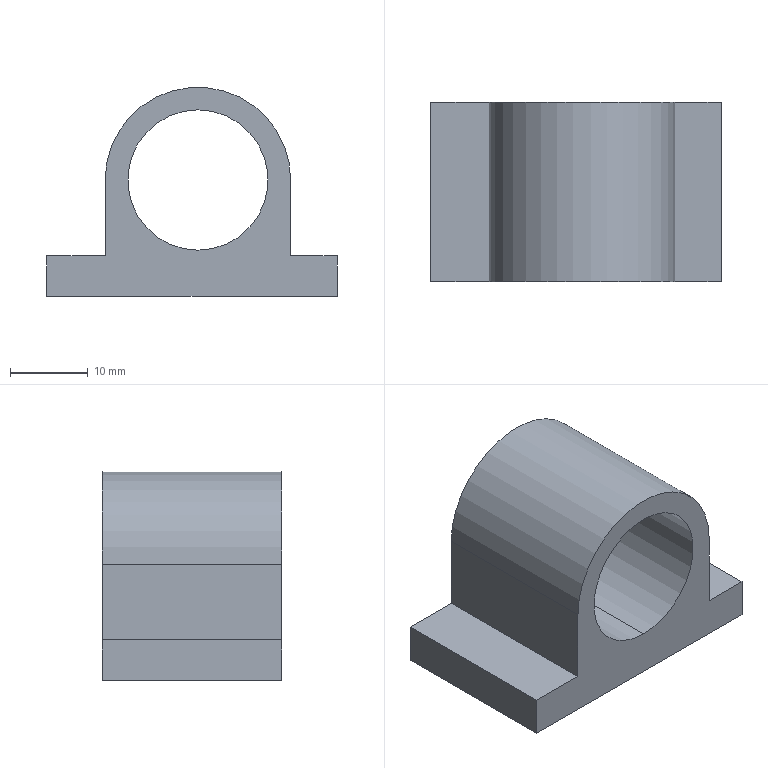Part | STEP file | 1 solid | 12 faces | box 37.23 x 23 x 26.824 mm | volume 9039 mm3 | plane 9 | cylinder 3 | commonest cylinder face diameters 18 x2 23.807 x1
STEP:
#1=CARTESIAN_POINT('',(0.,0.,0.));
#2=DIRECTION('',(0.,0.,1.));
#3=DIRECTION('',(1.,0.,0.));
#4=AXIS2_PLACEMENT_3D('',#1,#2,#3);
#5=CARTESIAN_POINT('',(340.649,373.299,152.933));
#6=VERTEX_POINT('',#5);
#7=CARTESIAN_POINT('',(340.649,350.299,152.933));
#8=VERTEX_POINT('',#7);
#9=CARTESIAN_POINT('',(340.649,373.299,152.933));
#10=DIRECTION('',(0.,-1.,0.));
#11=VECTOR('',#10,1.);
#12=LINE('',#9,#11);
#13=CARTESIAN_POINT('',(340.649,373.299,161.933));
#14=DIRECTION('',(0.,-1.,0.));
#15=DIRECTION('',(0.,0.,-1.));
#16=AXIS2_PLACEMENT_3D('',#13,#14,#15);
#17=CYLINDRICAL_SURFACE('',#16,9.);
#18=CARTESIAN_POINT('',(6.283,0.));
#19=DIRECTION('',(0.,1.));
#20=VECTOR('',#19,1.);
#21=LINE('',#18,#20);
#22=(GEOMETRIC_REPRESENTATION_CONTEXT(2)PARAMETRIC_REPRESENTATION_CONTEXT()REPRESENTATION_CONTEXT('',''));
#23=DEFINITIONAL_REPRESENTATION('',(#21),#22);
#24=PCURVE('',#17,#23);
#25=CARTESIAN_POINT('',(340.649,373.299,161.933));
#26=DIRECTION('',(0.,-1.,0.));
#27=DIRECTION('',(0.,0.,-1.));
#28=AXIS2_PLACEMENT_3D('',#25,#26,#27);
#29=CYLINDRICAL_SURFACE('',#28,9.);
#30=CARTESIAN_POINT('',(0.,0.));
#31=DIRECTION('',(0.,1.));
#32=VECTOR('',#31,1.);
#33=LINE('',#30,#32);
#34=(GEOMETRIC_REPRESENTATION_CONTEXT(2)PARAMETRIC_REPRESENTATION_CONTEXT()REPRESENTATION_CONTEXT('',''));
#35=DEFINITIONAL_REPRESENTATION('',(#33),#34);
#36=PCURVE('',#29,#35);
#37=SURFACE_CURVE('',#12,(#24,#36),.PCURVE_S1.);
#38=EDGE_CURVE('',#6,#8,#37,.T.);
#39=ORIENTED_EDGE('',*,*,#38,.T.);
#40=CARTESIAN_POINT('',(340.649,350.299,170.933));
#41=VERTEX_POINT('',#40);
#42=CARTESIAN_POINT('',(340.649,350.299,161.933));
#43=DIRECTION('',(0.,-1.,0.));
#44=DIRECTION('',(0.,0.,-1.));
#45=AXIS2_PLACEMENT_3D('',#42,#43,#44);
#46=CIRCLE('',#45,9.);
#47=CARTESIAN_POINT('',(0.,23.));
#48=DIRECTION('',(1.,0.));
#49=VECTOR('',#48,1.);
#50=LINE('',#47,#49);
#51=(GEOMETRIC_REPRESENTATION_CONTEXT(2)PARAMETRIC_REPRESENTATION_CONTEXT()REPRESENTATION_CONTEXT('',''));
#52=DEFINITIONAL_REPRESENTATION('',(#50),#51);
#53=PCURVE('',#17,#52);
#54=CARTESIAN_POINT('',(340.649,350.299,161.933));
#55=DIRECTION('',(0.,-1.,0.));
#56=DIRECTION('',(0.,0.,-1.));
#57=AXIS2_PLACEMENT_3D('',#54,#55,#56);
#58=PLANE('',#57);
#59=CARTESIAN_POINT('',(0.,0.));
#60=DIRECTION('',(1.,0.));
#61=AXIS2_PLACEMENT_2D('',#59,#60);
#62=CIRCLE('',#61,9.);
#63=(GEOMETRIC_REPRESENTATION_CONTEXT(2)PARAMETRIC_REPRESENTATION_CONTEXT()REPRESENTATION_CONTEXT('',''));
#64=DEFINITIONAL_REPRESENTATION('',(#62),#63);
#65=PCURVE('',#58,#64);
#66=SURFACE_CURVE('',#46,(#53,#65),.PCURVE_S1.);
#67=EDGE_CURVE('',#41,#8,#66,.T.);
#68=ORIENTED_EDGE('',*,*,#67,.F.);
#69=CARTESIAN_POINT('',(340.649,373.299,170.933));
#70=VERTEX_POINT('',#69);
#71=CARTESIAN_POINT('',(340.649,373.299,170.933));
#72=DIRECTION('',(0.,-1.,0.));
#73=VECTOR('',#72,1.);
#74=LINE('',#71,#73);
#75=CARTESIAN_POINT('',(3.142,0.));
#76=DIRECTION('',(0.,1.));
#77=VECTOR('',#76,1.);
#78=LINE('',#75,#77);
#79=(GEOMETRIC_REPRESENTATION_CONTEXT(2)PARAMETRIC_REPRESENTATION_CONTEXT()REPRESENTATION_CONTEXT('',''));
#80=DEFINITIONAL_REPRESENTATION('',(#78),#79);
#81=PCURVE('',#17,#80);
#82=CARTESIAN_POINT('',(3.142,0.));
#83=DIRECTION('',(0.,1.));
#84=VECTOR('',#83,1.);
#85=LINE('',#82,#84);
#86=(GEOMETRIC_REPRESENTATION_CONTEXT(2)PARAMETRIC_REPRESENTATION_CONTEXT()REPRESENTATION_CONTEXT('',''));
#87=DEFINITIONAL_REPRESENTATION('',(#85),#86);
#88=PCURVE('',#29,#87);
#89=SURFACE_CURVE('',#74,(#81,#88),.PCURVE_S1.);
#90=EDGE_CURVE('',#70,#41,#89,.T.);
#91=ORIENTED_EDGE('',*,*,#90,.F.);
#92=CARTESIAN_POINT('',(340.649,373.299,161.933));
#93=DIRECTION('',(0.,-1.,0.));
#94=DIRECTION('',(0.,0.,-1.));
#95=AXIS2_PLACEMENT_3D('',#92,#93,#94);
#96=CIRCLE('',#95,9.);
#97=CARTESIAN_POINT('',(0.,0.));
#98=DIRECTION('',(1.,0.));
#99=VECTOR('',#98,1.);
#100=LINE('',#97,#99);
#101=(GEOMETRIC_REPRESENTATION_CONTEXT(2)PARAMETRIC_REPRESENTATION_CONTEXT()REPRESENTATION_CONTEXT('',''));
#102=DEFINITIONAL_REPRESENTATION('',(#100),#101);
#103=PCURVE('',#17,#102);
#104=CARTESIAN_POINT('',(340.649,373.299,161.933));
#105=DIRECTION('',(0.,-1.,0.));
#106=DIRECTION('',(0.,0.,-1.));
#107=AXIS2_PLACEMENT_3D('',#104,#105,#106);
#108=PLANE('',#107);
#109=CARTESIAN_POINT('',(0.,0.));
#110=DIRECTION('',(1.,0.));
#111=AXIS2_PLACEMENT_2D('',#109,#110);
#112=CIRCLE('',#111,9.);
#113=(GEOMETRIC_REPRESENTATION_CONTEXT(2)PARAMETRIC_REPRESENTATION_CONTEXT()REPRESENTATION_CONTEXT('',''));
#114=DEFINITIONAL_REPRESENTATION('',(#112),#113);
#115=PCURVE('',#108,#114);
#116=SURFACE_CURVE('',#96,(#103,#115),.PCURVE_S1.);
#117=EDGE_CURVE('',#70,#6,#116,.T.);
#118=ORIENTED_EDGE('',*,*,#117,.T.);
#119=EDGE_LOOP('',(#39,#68,#91,#118));
#120=FACE_BOUND('',#119,.F.);
#121=ADVANCED_FACE('',(#120),#17,.F.);
#122=CARTESIAN_POINT('',(321.271,350.299,152.204));
#123=VERTEX_POINT('',#122);
#124=CARTESIAN_POINT('',(321.271,350.299,147.013));
#125=VERTEX_POINT('',#124);
#126=CARTESIAN_POINT('',(321.271,350.299,147.013));
#127=DIRECTION('',(0.,0.,-1.));
#128=VECTOR('',#127,1.);
#129=LINE('',#126,#128);
#130=CARTESIAN_POINT('',(321.271,373.299,147.013));
#131=DIRECTION('',(-1.,0.,0.));
#132=DIRECTION('',(0.,0.,1.));
#133=AXIS2_PLACEMENT_3D('',#130,#131,#132);
#134=PLANE('',#133);
#135=CARTESIAN_POINT('',(0.,-23.));
#136=DIRECTION('',(-1.,0.));
#137=VECTOR('',#136,1.);
#138=LINE('',#135,#137);
#139=(GEOMETRIC_REPRESENTATION_CONTEXT(2)PARAMETRIC_REPRESENTATION_CONTEXT()REPRESENTATION_CONTEXT('',''));
#140=DEFINITIONAL_REPRESENTATION('',(#138),#139);
#141=PCURVE('',#134,#140);
#142=CARTESIAN_POINT('',(14.921,-19.377));
#143=DIRECTION('',(1.,0.));
#144=VECTOR('',#143,1.);
#145=LINE('',#142,#144);
#146=(GEOMETRIC_REPRESENTATION_CONTEXT(2)PARAMETRIC_REPRESENTATION_CONTEXT()REPRESENTATION_CONTEXT('',''));
#147=DEFINITIONAL_REPRESENTATION('',(#145),#146);
#148=PCURVE('',#58,#147);
#149=SURFACE_CURVE('',#129,(#141,#148),.PCURVE_S1.);
#150=EDGE_CURVE('',#123,#125,#149,.T.);
#151=ORIENTED_EDGE('',*,*,#150,.F.);
#152=CARTESIAN_POINT('',(321.271,373.299,152.204));
#153=VERTEX_POINT('',#152);
#154=CARTESIAN_POINT('',(321.271,373.299,152.204));
#155=DIRECTION('',(0.,-1.,0.));
#156=VECTOR('',#155,1.);
#157=LINE('',#154,#156);
#158=CARTESIAN_POINT('',(5.191,0.));
#159=DIRECTION('',(0.,-1.));
#160=VECTOR('',#159,1.);
#161=LINE('',#158,#160);
#162=(GEOMETRIC_REPRESENTATION_CONTEXT(2)PARAMETRIC_REPRESENTATION_CONTEXT()REPRESENTATION_CONTEXT('',''));
#163=DEFINITIONAL_REPRESENTATION('',(#161),#162);
#164=PCURVE('',#134,#163);
#165=CARTESIAN_POINT('',(321.271,373.299,152.204));
#166=DIRECTION('',(0.,0.,1.));
#167=DIRECTION('',(1.,0.,0.));
#168=AXIS2_PLACEMENT_3D('',#165,#166,#167);
#169=PLANE('',#168);
#170=CARTESIAN_POINT('',(0.,0.));
#171=DIRECTION('',(0.,-1.));
#172=VECTOR('',#171,1.);
#173=LINE('',#170,#172);
#174=(GEOMETRIC_REPRESENTATION_CONTEXT(2)PARAMETRIC_REPRESENTATION_CONTEXT()REPRESENTATION_CONTEXT('',''));
#175=DEFINITIONAL_REPRESENTATION('',(#173),#174);
#176=PCURVE('',#169,#175);
#177=SURFACE_CURVE('',#157,(#164,#176),.PCURVE_S1.);
#178=EDGE_CURVE('',#153,#123,#177,.T.);
#179=ORIENTED_EDGE('',*,*,#178,.F.);
#180=CARTESIAN_POINT('',(321.271,373.299,147.013));
#181=VERTEX_POINT('',#180);
#182=CARTESIAN_POINT('',(321.271,373.299,147.013));
#183=DIRECTION('',(0.,0.,-1.));
#184=VECTOR('',#183,1.);
#185=LINE('',#182,#184);
#186=CARTESIAN_POINT('',(0.,0.));
#187=DIRECTION('',(-1.,0.));
#188=VECTOR('',#187,1.);
#189=LINE('',#186,#188);
#190=(GEOMETRIC_REPRESENTATION_CONTEXT(2)PARAMETRIC_REPRESENTATION_CONTEXT()REPRESENTATION_CONTEXT('',''));
#191=DEFINITIONAL_REPRESENTATION('',(#189),#190);
#192=PCURVE('',#134,#191);
#193=CARTESIAN_POINT('',(14.921,-19.377));
#194=DIRECTION('',(1.,0.));
#195=VECTOR('',#194,1.);
#196=LINE('',#193,#195);
#197=(GEOMETRIC_REPRESENTATION_CONTEXT(2)PARAMETRIC_REPRESENTATION_CONTEXT()REPRESENTATION_CONTEXT('',''));
#198=DEFINITIONAL_REPRESENTATION('',(#196),#197);
#199=PCURVE('',#108,#198);
#200=SURFACE_CURVE('',#185,(#192,#199),.PCURVE_S1.);
#201=EDGE_CURVE('',#153,#181,#200,.T.);
#202=ORIENTED_EDGE('',*,*,#201,.T.);
#203=CARTESIAN_POINT('',(321.271,373.299,147.013));
#204=DIRECTION('',(0.,-1.,0.));
#205=VECTOR('',#204,1.);
#206=LINE('',#203,#205);
#207=CARTESIAN_POINT('',(0.,0.));
#208=DIRECTION('',(0.,-1.));
#209=VECTOR('',#208,1.);
#210=LINE('',#207,#209);
#211=(GEOMETRIC_REPRESENTATION_CONTEXT(2)PARAMETRIC_REPRESENTATION_CONTEXT()REPRESENTATION_CONTEXT('',''));
#212=DEFINITIONAL_REPRESENTATION('',(#210),#211);
#213=PCURVE('',#134,#212);
#214=CARTESIAN_POINT('',(321.271,373.299,147.013));
#215=DIRECTION('',(0.,0.,-1.));
#216=DIRECTION('',(-1.,0.,0.));
#217=AXIS2_PLACEMENT_3D('',#214,#215,#216);
#218=PLANE('',#217);
#219=CARTESIAN_POINT('',(0.,0.));
#220=DIRECTION('',(0.,-1.));
#221=VECTOR('',#220,1.);
#222=LINE('',#219,#221);
#223=(GEOMETRIC_REPRESENTATION_CONTEXT(2)PARAMETRIC_REPRESENTATION_CONTEXT()REPRESENTATION_CONTEXT('',''));
#224=DEFINITIONAL_REPRESENTATION('',(#222),#223);
#225=PCURVE('',#218,#224);
#226=SURFACE_CURVE('',#206,(#213,#225),.PCURVE_S1.);
#227=EDGE_CURVE('',#181,#125,#226,.T.);
#228=ORIENTED_EDGE('',*,*,#227,.T.);
#229=EDGE_LOOP('',(#151,#179,#202,#228));
#230=FACE_BOUND('',#229,.T.);
#231=ADVANCED_FACE('',(#230),#134,.T.);
#232=CARTESIAN_POINT('',(328.745,350.299,152.204));
#233=VERTEX_POINT('',#232);
#234=CARTESIAN_POINT('',(321.271,350.299,152.204));
#235=DIRECTION('',(-1.,0.,0.));
#236=VECTOR('',#235,1.);
#237=LINE('',#234,#236);
#238=CARTESIAN_POINT('',(0.,-23.));
#239=DIRECTION('',(-1.,0.));
#240=VECTOR('',#239,1.);
#241=LINE('',#238,#240);
#242=(GEOMETRIC_REPRESENTATION_CONTEXT(2)PARAMETRIC_REPRESENTATION_CONTEXT()REPRESENTATION_CONTEXT('',''));
#243=DEFINITIONAL_REPRESENTATION('',(#241),#242);
#244=PCURVE('',#169,#243);
#245=CARTESIAN_POINT('',(9.73,-19.377));
#246=DIRECTION('',(0.,-1.));
#247=VECTOR('',#246,1.);
#248=LINE('',#245,#247);
#249=(GEOMETRIC_REPRESENTATION_CONTEXT(2)PARAMETRIC_REPRESENTATION_CONTEXT()REPRESENTATION_CONTEXT('',''));
#250=DEFINITIONAL_REPRESENTATION('',(#248),#249);
#251=PCURVE('',#58,#250);
#252=SURFACE_CURVE('',#237,(#244,#251),.PCURVE_S1.);
#253=EDGE_CURVE('',#233,#123,#252,.T.);
#254=ORIENTED_EDGE('',*,*,#253,.F.);
#255=CARTESIAN_POINT('',(328.745,373.299,152.204));
#256=VERTEX_POINT('',#255);
#257=CARTESIAN_POINT('',(328.745,373.299,152.204));
#258=DIRECTION('',(0.,-1.,0.));
#259=VECTOR('',#258,1.);
#260=LINE('',#257,#259);
#261=CARTESIAN_POINT('',(7.474,0.));
#262=DIRECTION('',(0.,-1.));
#263=VECTOR('',#262,1.);
#264=LINE('',#261,#263);
#265=(GEOMETRIC_REPRESENTATION_CONTEXT(2)PARAMETRIC_REPRESENTATION_CONTEXT()REPRESENTATION_CONTEXT('',''));
#266=DEFINITIONAL_REPRESENTATION('',(#264),#265);
#267=PCURVE('',#169,#266);
#268=CARTESIAN_POINT('',(328.745,373.299,161.933));
#269=DIRECTION('',(-1.,0.,0.));
#270=DIRECTION('',(0.,0.,1.));
#271=AXIS2_PLACEMENT_3D('',#268,#269,#270);
#272=PLANE('',#271);
#273=CARTESIAN_POINT('',(-9.73,0.));
#274=DIRECTION('',(0.,-1.));
#275=VECTOR('',#274,1.);
#276=LINE('',#273,#275);
#277=(GEOMETRIC_REPRESENTATION_CONTEXT(2)PARAMETRIC_REPRESENTATION_CONTEXT()REPRESENTATION_CONTEXT('',''));
#278=DEFINITIONAL_REPRESENTATION('',(#276),#277);
#279=PCURVE('',#272,#278);
#280=SURFACE_CURVE('',#260,(#267,#279),.PCURVE_S1.);
#281=EDGE_CURVE('',#256,#233,#280,.T.);
#282=ORIENTED_EDGE('',*,*,#281,.F.);
#283=CARTESIAN_POINT('',(321.271,373.299,152.204));
#284=DIRECTION('',(-1.,0.,0.));
#285=VECTOR('',#284,1.);
#286=LINE('',#283,#285);
#287=CARTESIAN_POINT('',(0.,0.));
#288=DIRECTION('',(-1.,0.));
#289=VECTOR('',#288,1.);
#290=LINE('',#287,#289);
#291=(GEOMETRIC_REPRESENTATION_CONTEXT(2)PARAMETRIC_REPRESENTATION_CONTEXT()REPRESENTATION_CONTEXT('',''));
#292=DEFINITIONAL_REPRESENTATION('',(#290),#291);
#293=PCURVE('',#169,#292);
#294=CARTESIAN_POINT('',(9.73,-19.377));
#295=DIRECTION('',(0.,-1.));
#296=VECTOR('',#295,1.);
#297=LINE('',#294,#296);
#298=(GEOMETRIC_REPRESENTATION_CONTEXT(2)PARAMETRIC_REPRESENTATION_CONTEXT()REPRESENTATION_CONTEXT('',''));
#299=DEFINITIONAL_REPRESENTATION('',(#297),#298);
#300=PCURVE('',#108,#299);
#301=SURFACE_CURVE('',#286,(#293,#300),.PCURVE_S1.);
#302=EDGE_CURVE('',#256,#153,#301,.T.);
#303=ORIENTED_EDGE('',*,*,#302,.T.);
#304=ORIENTED_EDGE('',*,*,#178,.T.);
#305=EDGE_LOOP('',(#254,#282,#303,#304));
#306=FACE_BOUND('',#305,.T.);
#307=ADVANCED_FACE('',(#306),#169,.T.);
#308=CARTESIAN_POINT('',(328.745,350.299,161.933));
#309=VERTEX_POINT('',#308);
#310=CARTESIAN_POINT('',(328.745,350.299,161.933));
#311=DIRECTION('',(0.,0.,-1.));
#312=VECTOR('',#311,1.);
#313=LINE('',#310,#312);
#314=CARTESIAN_POINT('',(0.,-23.));
#315=DIRECTION('',(-1.,0.));
#316=VECTOR('',#315,1.);
#317=LINE('',#314,#316);
#318=(GEOMETRIC_REPRESENTATION_CONTEXT(2)PARAMETRIC_REPRESENTATION_CONTEXT()REPRESENTATION_CONTEXT('',''));
#319=DEFINITIONAL_REPRESENTATION('',(#317),#318);
#320=PCURVE('',#272,#319);
#321=CARTESIAN_POINT('',(0.,-11.903));
#322=DIRECTION('',(1.,0.));
#323=VECTOR('',#322,1.);
#324=LINE('',#321,#323);
#325=(GEOMETRIC_REPRESENTATION_CONTEXT(2)PARAMETRIC_REPRESENTATION_CONTEXT()REPRESENTATION_CONTEXT('',''));
#326=DEFINITIONAL_REPRESENTATION('',(#324),#325);
#327=PCURVE('',#58,#326);
#328=SURFACE_CURVE('',#313,(#320,#327),.PCURVE_S1.);
#329=EDGE_CURVE('',#309,#233,#328,.T.);
#330=ORIENTED_EDGE('',*,*,#329,.F.);
#331=CARTESIAN_POINT('',(328.745,373.299,161.933));
#332=VERTEX_POINT('',#331);
#333=CARTESIAN_POINT('',(328.745,373.299,161.933));
#334=DIRECTION('',(0.,-1.,0.));
#335=VECTOR('',#334,1.);
#336=LINE('',#333,#335);
#337=CARTESIAN_POINT('',(0.,0.));
#338=DIRECTION('',(0.,-1.));
#339=VECTOR('',#338,1.);
#340=LINE('',#337,#339);
#341=(GEOMETRIC_REPRESENTATION_CONTEXT(2)PARAMETRIC_REPRESENTATION_CONTEXT()REPRESENTATION_CONTEXT('',''));
#342=DEFINITIONAL_REPRESENTATION('',(#340),#341);
#343=PCURVE('',#272,#342);
#344=CARTESIAN_POINT('',(340.649,373.299,161.933));
#345=DIRECTION('',(0.,-1.,0.));
#346=DIRECTION('',(0.,0.,-1.));
#347=AXIS2_PLACEMENT_3D('',#344,#345,#346);
#348=CYLINDRICAL_SURFACE('',#347,11.903);
#349=CARTESIAN_POINT('',(4.712,0.));
#350=DIRECTION('',(0.,1.));
#351=VECTOR('',#350,1.);
#352=LINE('',#349,#351);
#353=(GEOMETRIC_REPRESENTATION_CONTEXT(2)PARAMETRIC_REPRESENTATION_CONTEXT()REPRESENTATION_CONTEXT('',''));
#354=DEFINITIONAL_REPRESENTATION('',(#352),#353);
#355=PCURVE('',#348,#354);
#356=SURFACE_CURVE('',#336,(#343,#355),.PCURVE_S1.);
#357=EDGE_CURVE('',#332,#309,#356,.T.);
#358=ORIENTED_EDGE('',*,*,#357,.F.);
#359=CARTESIAN_POINT('',(328.745,373.299,161.933));
#360=DIRECTION('',(0.,0.,-1.));
#361=VECTOR('',#360,1.);
#362=LINE('',#359,#361);
#363=CARTESIAN_POINT('',(0.,0.));
#364=DIRECTION('',(-1.,0.));
#365=VECTOR('',#364,1.);
#366=LINE('',#363,#365);
#367=(GEOMETRIC_REPRESENTATION_CONTEXT(2)PARAMETRIC_REPRESENTATION_CONTEXT()REPRESENTATION_CONTEXT('',''));
#368=DEFINITIONAL_REPRESENTATION('',(#366),#367);
#369=PCURVE('',#272,#368);
#370=CARTESIAN_POINT('',(0.,-11.903));
#371=DIRECTION('',(1.,0.));
#372=VECTOR('',#371,1.);
#373=LINE('',#370,#372);
#374=(GEOMETRIC_REPRESENTATION_CONTEXT(2)PARAMETRIC_REPRESENTATION_CONTEXT()REPRESENTATION_CONTEXT('',''));
#375=DEFINITIONAL_REPRESENTATION('',(#373),#374);
#376=PCURVE('',#108,#375);
#377=SURFACE_CURVE('',#362,(#369,#376),.PCURVE_S1.);
#378=EDGE_CURVE('',#332,#256,#377,.T.);
#379=ORIENTED_EDGE('',*,*,#378,.T.);
#380=ORIENTED_EDGE('',*,*,#281,.T.);
#381=EDGE_LOOP('',(#330,#358,#379,#380));
#382=FACE_BOUND('',#381,.T.);
#383=ADVANCED_FACE('',(#382),#272,.T.);
#384=CARTESIAN_POINT('',(352.552,350.299,161.933));
#385=VERTEX_POINT('',#384);
#386=CARTESIAN_POINT('',(340.649,350.299,161.933));
#387=DIRECTION('',(0.,-1.,0.));
#388=DIRECTION('',(0.,0.,-1.));
#389=AXIS2_PLACEMENT_3D('',#386,#387,#388);
#390=CIRCLE('',#389,11.903);
#391=CARTESIAN_POINT('',(0.,23.));
#392=DIRECTION('',(1.,0.));
#393=VECTOR('',#392,1.);
#394=LINE('',#391,#393);
#395=(GEOMETRIC_REPRESENTATION_CONTEXT(2)PARAMETRIC_REPRESENTATION_CONTEXT()REPRESENTATION_CONTEXT('',''));
#396=DEFINITIONAL_REPRESENTATION('',(#394),#395);
#397=PCURVE('',#348,#396);
#398=CARTESIAN_POINT('',(0.,0.));
#399=DIRECTION('',(1.,0.));
#400=AXIS2_PLACEMENT_2D('',#398,#399);
#401=CIRCLE('',#400,11.903);
#402=(GEOMETRIC_REPRESENTATION_CONTEXT(2)PARAMETRIC_REPRESENTATION_CONTEXT()REPRESENTATION_CONTEXT('',''));
#403=DEFINITIONAL_REPRESENTATION('',(#401),#402);
#404=PCURVE('',#58,#403);
#405=SURFACE_CURVE('',#390,(#397,#404),.PCURVE_S1.);
#406=EDGE_CURVE('',#385,#309,#405,.T.);
#407=ORIENTED_EDGE('',*,*,#406,.F.);
#408=CARTESIAN_POINT('',(352.552,373.299,161.933));
#409=VERTEX_POINT('',#408);
#410=CARTESIAN_POINT('',(352.552,373.299,161.933));
#411=DIRECTION('',(0.,-1.,0.));
#412=VECTOR('',#411,1.);
#413=LINE('',#410,#412);
#414=CARTESIAN_POINT('',(1.571,0.));
#415=DIRECTION('',(0.,1.));
#416=VECTOR('',#415,1.);
#417=LINE('',#414,#416);
#418=(GEOMETRIC_REPRESENTATION_CONTEXT(2)PARAMETRIC_REPRESENTATION_CONTEXT()REPRESENTATION_CONTEXT('',''));
#419=DEFINITIONAL_REPRESENTATION('',(#417),#418);
#420=PCURVE('',#348,#419);
#421=CARTESIAN_POINT('',(352.552,373.299,161.933));
#422=DIRECTION('',(1.,0.,0.));
#423=DIRECTION('',(0.,0.,-1.));
#424=AXIS2_PLACEMENT_3D('',#421,#422,#423);
#425=PLANE('',#424);
#426=CARTESIAN_POINT('',(0.,0.));
#427=DIRECTION('',(0.,-1.));
#428=VECTOR('',#427,1.);
#429=LINE('',#426,#428);
#430=(GEOMETRIC_REPRESENTATION_CONTEXT(2)PARAMETRIC_REPRESENTATION_CONTEXT()REPRESENTATION_CONTEXT('',''));
#431=DEFINITIONAL_REPRESENTATION('',(#429),#430);
#432=PCURVE('',#425,#431);
#433=SURFACE_CURVE('',#413,(#420,#432),.PCURVE_S1.);
#434=EDGE_CURVE('',#409,#385,#433,.T.);
#435=ORIENTED_EDGE('',*,*,#434,.F.);
#436=CARTESIAN_POINT('',(340.649,373.299,161.933));
#437=DIRECTION('',(0.,-1.,0.));
#438=DIRECTION('',(0.,0.,-1.));
#439=AXIS2_PLACEMENT_3D('',#436,#437,#438);
#440=CIRCLE('',#439,11.903);
#441=CARTESIAN_POINT('',(0.,0.));
#442=DIRECTION('',(1.,0.));
#443=VECTOR('',#442,1.);
#444=LINE('',#441,#443);
#445=(GEOMETRIC_REPRESENTATION_CONTEXT(2)PARAMETRIC_REPRESENTATION_CONTEXT()REPRESENTATION_CONTEXT('',''));
#446=DEFINITIONAL_REPRESENTATION('',(#444),#445);
#447=PCURVE('',#348,#446);
#448=CARTESIAN_POINT('',(0.,0.));
#449=DIRECTION('',(1.,0.));
#450=AXIS2_PLACEMENT_2D('',#448,#449);
#451=CIRCLE('',#450,11.903);
#452=(GEOMETRIC_REPRESENTATION_CONTEXT(2)PARAMETRIC_REPRESENTATION_CONTEXT()REPRESENTATION_CONTEXT('',''));
#453=DEFINITIONAL_REPRESENTATION('',(#451),#452);
#454=PCURVE('',#108,#453);
#455=SURFACE_CURVE('',#440,(#447,#454),.PCURVE_S1.);
#456=EDGE_CURVE('',#409,#332,#455,.T.);
#457=ORIENTED_EDGE('',*,*,#456,.T.);
#458=ORIENTED_EDGE('',*,*,#357,.T.);
#459=EDGE_LOOP('',(#407,#435,#457,#458));
#460=FACE_BOUND('',#459,.T.);
#461=ADVANCED_FACE('',(#460),#348,.T.);
#462=CARTESIAN_POINT('',(352.552,350.299,152.204));
#463=VERTEX_POINT('',#462);
#464=CARTESIAN_POINT('',(352.552,350.299,161.933));
#465=DIRECTION('',(0.,0.,1.));
#466=VECTOR('',#465,1.);
#467=LINE('',#464,#466);
#468=CARTESIAN_POINT('',(0.,-23.));
#469=DIRECTION('',(-1.,0.));
#470=VECTOR('',#469,1.);
#471=LINE('',#468,#470);
#472=(GEOMETRIC_REPRESENTATION_CONTEXT(2)PARAMETRIC_REPRESENTATION_CONTEXT()REPRESENTATION_CONTEXT('',''));
#473=DEFINITIONAL_REPRESENTATION('',(#471),#472);
#474=PCURVE('',#425,#473);
#475=CARTESIAN_POINT('',(0.,11.903));
#476=DIRECTION('',(-1.,0.));
#477=VECTOR('',#476,1.);
#478=LINE('',#475,#477);
#479=(GEOMETRIC_REPRESENTATION_CONTEXT(2)PARAMETRIC_REPRESENTATION_CONTEXT()REPRESENTATION_CONTEXT('',''));
#480=DEFINITIONAL_REPRESENTATION('',(#478),#479);
#481=PCURVE('',#58,#480);
#482=SURFACE_CURVE('',#467,(#474,#481),.PCURVE_S1.);
#483=EDGE_CURVE('',#463,#385,#482,.T.);
#484=ORIENTED_EDGE('',*,*,#483,.F.);
#485=CARTESIAN_POINT('',(352.552,373.299,152.204));
#486=VERTEX_POINT('',#485);
#487=CARTESIAN_POINT('',(352.552,373.299,152.204));
#488=DIRECTION('',(0.,-1.,0.));
#489=VECTOR('',#488,1.);
#490=LINE('',#487,#489);
#491=CARTESIAN_POINT('',(9.73,0.));
#492=DIRECTION('',(0.,-1.));
#493=VECTOR('',#492,1.);
#494=LINE('',#491,#493);
#495=(GEOMETRIC_REPRESENTATION_CONTEXT(2)PARAMETRIC_REPRESENTATION_CONTEXT()REPRESENTATION_CONTEXT('',''));
#496=DEFINITIONAL_REPRESENTATION('',(#494),#495);
#497=PCURVE('',#425,#496);
#498=CARTESIAN_POINT('',(352.552,373.299,152.204));
#499=DIRECTION('',(0.,0.,1.));
#500=DIRECTION('',(1.,0.,0.));
#501=AXIS2_PLACEMENT_3D('',#498,#499,#500);
#502=PLANE('',#501);
#503=CARTESIAN_POINT('',(0.,0.));
#504=DIRECTION('',(0.,-1.));
#505=VECTOR('',#504,1.);
#506=LINE('',#503,#505);
#507=(GEOMETRIC_REPRESENTATION_CONTEXT(2)PARAMETRIC_REPRESENTATION_CONTEXT()REPRESENTATION_CONTEXT('',''));
#508=DEFINITIONAL_REPRESENTATION('',(#506),#507);
#509=PCURVE('',#502,#508);
#510=SURFACE_CURVE('',#490,(#497,#509),.PCURVE_S1.);
#511=EDGE_CURVE('',#486,#463,#510,.T.);
#512=ORIENTED_EDGE('',*,*,#511,.F.);
#513=CARTESIAN_POINT('',(352.552,373.299,161.933));
#514=DIRECTION('',(0.,0.,1.));
#515=VECTOR('',#514,1.);
#516=LINE('',#513,#515);
#517=CARTESIAN_POINT('',(0.,0.));
#518=DIRECTION('',(-1.,0.));
#519=VECTOR('',#518,1.);
#520=LINE('',#517,#519);
#521=(GEOMETRIC_REPRESENTATION_CONTEXT(2)PARAMETRIC_REPRESENTATION_CONTEXT()REPRESENTATION_CONTEXT('',''));
#522=DEFINITIONAL_REPRESENTATION('',(#520),#521);
#523=PCURVE('',#425,#522);
#524=CARTESIAN_POINT('',(0.,11.903));
#525=DIRECTION('',(-1.,0.));
#526=VECTOR('',#525,1.);
#527=LINE('',#524,#526);
#528=(GEOMETRIC_REPRESENTATION_CONTEXT(2)PARAMETRIC_REPRESENTATION_CONTEXT()REPRESENTATION_CONTEXT('',''));
#529=DEFINITIONAL_REPRESENTATION('',(#527),#528);
#530=PCURVE('',#108,#529);
#531=SURFACE_CURVE('',#516,(#523,#530),.PCURVE_S1.);
#532=EDGE_CURVE('',#486,#409,#531,.T.);
#533=ORIENTED_EDGE('',*,*,#532,.T.);
#534=ORIENTED_EDGE('',*,*,#434,.T.);
#535=EDGE_LOOP('',(#484,#512,#533,#534));
#536=FACE_BOUND('',#535,.T.);
#537=ADVANCED_FACE('',(#536),#425,.T.);
#538=CARTESIAN_POINT('',(358.501,350.299,152.204));
#539=VERTEX_POINT('',#538);
#540=CARTESIAN_POINT('',(352.552,350.299,152.204));
#541=DIRECTION('',(-1.,0.,0.));
#542=VECTOR('',#541,1.);
#543=LINE('',#540,#542);
#544=CARTESIAN_POINT('',(0.,-23.));
#545=DIRECTION('',(-1.,0.));
#546=VECTOR('',#545,1.);
#547=LINE('',#544,#546);
#548=(GEOMETRIC_REPRESENTATION_CONTEXT(2)PARAMETRIC_REPRESENTATION_CONTEXT()REPRESENTATION_CONTEXT('',''));
#549=DEFINITIONAL_REPRESENTATION('',(#547),#548);
#550=PCURVE('',#502,#549);
#551=CARTESIAN_POINT('',(9.73,11.903));
#552=DIRECTION('',(0.,-1.));
#553=VECTOR('',#552,1.);
#554=LINE('',#551,#553);
#555=(GEOMETRIC_REPRESENTATION_CONTEXT(2)PARAMETRIC_REPRESENTATION_CONTEXT()REPRESENTATION_CONTEXT('',''));
#556=DEFINITIONAL_REPRESENTATION('',(#554),#555);
#557=PCURVE('',#58,#556);
#558=SURFACE_CURVE('',#543,(#550,#557),.PCURVE_S1.);
#559=EDGE_CURVE('',#539,#463,#558,.T.);
#560=ORIENTED_EDGE('',*,*,#559,.F.);
#561=CARTESIAN_POINT('',(358.501,373.299,152.204));
#562=VERTEX_POINT('',#561);
#563=CARTESIAN_POINT('',(358.501,373.299,152.204));
#564=DIRECTION('',(0.,-1.,0.));
#565=VECTOR('',#564,1.);
#566=LINE('',#563,#565);
#567=CARTESIAN_POINT('',(5.949,0.));
#568=DIRECTION('',(0.,-1.));
#569=VECTOR('',#568,1.);
#570=LINE('',#567,#569);
#571=(GEOMETRIC_REPRESENTATION_CONTEXT(2)PARAMETRIC_REPRESENTATION_CONTEXT()REPRESENTATION_CONTEXT('',''));
#572=DEFINITIONAL_REPRESENTATION('',(#570),#571);
#573=PCURVE('',#502,#572);
#574=CARTESIAN_POINT('',(358.501,373.299,147.013));
#575=DIRECTION('',(1.,0.,0.));
#576=DIRECTION('',(0.,0.,-1.));
#577=AXIS2_PLACEMENT_3D('',#574,#575,#576);
#578=PLANE('',#577);
#579=CARTESIAN_POINT('',(-5.191,0.));
#580=DIRECTION('',(0.,-1.));
#581=VECTOR('',#580,1.);
#582=LINE('',#579,#581);
#583=(GEOMETRIC_REPRESENTATION_CONTEXT(2)PARAMETRIC_REPRESENTATION_CONTEXT()REPRESENTATION_CONTEXT('',''));
#584=DEFINITIONAL_REPRESENTATION('',(#582),#583);
#585=PCURVE('',#578,#584);
#586=SURFACE_CURVE('',#566,(#573,#585),.PCURVE_S1.);
#587=EDGE_CURVE('',#562,#539,#586,.T.);
#588=ORIENTED_EDGE('',*,*,#587,.F.);
#589=CARTESIAN_POINT('',(352.552,373.299,152.204));
#590=DIRECTION('',(-1.,0.,0.));
#591=VECTOR('',#590,1.);
#592=LINE('',#589,#591);
#593=CARTESIAN_POINT('',(0.,0.));
#594=DIRECTION('',(-1.,0.));
#595=VECTOR('',#594,1.);
#596=LINE('',#593,#595);
#597=(GEOMETRIC_REPRESENTATION_CONTEXT(2)PARAMETRIC_REPRESENTATION_CONTEXT()REPRESENTATION_CONTEXT('',''));
#598=DEFINITIONAL_REPRESENTATION('',(#596),#597);
#599=PCURVE('',#502,#598);
#600=CARTESIAN_POINT('',(9.73,11.903));
#601=DIRECTION('',(0.,-1.));
#602=VECTOR('',#601,1.);
#603=LINE('',#600,#602);
#604=(GEOMETRIC_REPRESENTATION_CONTEXT(2)PARAMETRIC_REPRESENTATION_CONTEXT()REPRESENTATION_CONTEXT('',''));
#605=DEFINITIONAL_REPRESENTATION('',(#603),#604);
#606=PCURVE('',#108,#605);
#607=SURFACE_CURVE('',#592,(#599,#606),.PCURVE_S1.);
#608=EDGE_CURVE('',#562,#486,#607,.T.);
#609=ORIENTED_EDGE('',*,*,#608,.T.);
#610=ORIENTED_EDGE('',*,*,#511,.T.);
#611=EDGE_LOOP('',(#560,#588,#609,#610));
#612=FACE_BOUND('',#611,.T.);
#613=ADVANCED_FACE('',(#612),#502,.T.);
#614=CARTESIAN_POINT('',(358.501,350.299,147.013));
#615=VERTEX_POINT('',#614);
#616=CARTESIAN_POINT('',(358.501,350.299,147.013));
#617=DIRECTION('',(0.,0.,1.));
#618=VECTOR('',#617,1.);
#619=LINE('',#616,#618);
#620=CARTESIAN_POINT('',(0.,-23.));
#621=DIRECTION('',(-1.,0.));
#622=VECTOR('',#621,1.);
#623=LINE('',#620,#622);
#624=(GEOMETRIC_REPRESENTATION_CONTEXT(2)PARAMETRIC_REPRESENTATION_CONTEXT()REPRESENTATION_CONTEXT('',''));
#625=DEFINITIONAL_REPRESENTATION('',(#623),#624);
#626=PCURVE('',#578,#625);
#627=CARTESIAN_POINT('',(14.921,17.853));
#628=DIRECTION('',(-1.,0.));
#629=VECTOR('',#628,1.);
#630=LINE('',#627,#629);
#631=(GEOMETRIC_REPRESENTATION_CONTEXT(2)PARAMETRIC_REPRESENTATION_CONTEXT()REPRESENTATION_CONTEXT('',''));
#632=DEFINITIONAL_REPRESENTATION('',(#630),#631);
#633=PCURVE('',#58,#632);
#634=SURFACE_CURVE('',#619,(#626,#633),.PCURVE_S1.);
#635=EDGE_CURVE('',#615,#539,#634,.T.);
#636=ORIENTED_EDGE('',*,*,#635,.F.);
#637=CARTESIAN_POINT('',(358.501,373.299,147.013));
#638=VERTEX_POINT('',#637);
#639=CARTESIAN_POINT('',(358.501,373.299,147.013));
#640=DIRECTION('',(0.,-1.,0.));
#641=VECTOR('',#640,1.);
#642=LINE('',#639,#641);
#643=CARTESIAN_POINT('',(0.,0.));
#644=DIRECTION('',(0.,-1.));
#645=VECTOR('',#644,1.);
#646=LINE('',#643,#645);
#647=(GEOMETRIC_REPRESENTATION_CONTEXT(2)PARAMETRIC_REPRESENTATION_CONTEXT()REPRESENTATION_CONTEXT('',''));
#648=DEFINITIONAL_REPRESENTATION('',(#646),#647);
#649=PCURVE('',#578,#648);
#650=CARTESIAN_POINT('',(-37.23,0.));
#651=DIRECTION('',(0.,-1.));
#652=VECTOR('',#651,1.);
#653=LINE('',#650,#652);
#654=(GEOMETRIC_REPRESENTATION_CONTEXT(2)PARAMETRIC_REPRESENTATION_CONTEXT()REPRESENTATION_CONTEXT('',''));
#655=DEFINITIONAL_REPRESENTATION('',(#653),#654);
#656=PCURVE('',#218,#655);
#657=SURFACE_CURVE('',#642,(#649,#656),.PCURVE_S1.);
#658=EDGE_CURVE('',#638,#615,#657,.T.);
#659=ORIENTED_EDGE('',*,*,#658,.F.);
#660=CARTESIAN_POINT('',(358.501,373.299,147.013));
#661=DIRECTION('',(0.,0.,1.));
#662=VECTOR('',#661,1.);
#663=LINE('',#660,#662);
#664=CARTESIAN_POINT('',(0.,0.));
#665=DIRECTION('',(-1.,0.));
#666=VECTOR('',#665,1.);
#667=LINE('',#664,#666);
#668=(GEOMETRIC_REPRESENTATION_CONTEXT(2)PARAMETRIC_REPRESENTATION_CONTEXT()REPRESENTATION_CONTEXT('',''));
#669=DEFINITIONAL_REPRESENTATION('',(#667),#668);
#670=PCURVE('',#578,#669);
#671=CARTESIAN_POINT('',(14.921,17.853));
#672=DIRECTION('',(-1.,0.));
#673=VECTOR('',#672,1.);
#674=LINE('',#671,#673);
#675=(GEOMETRIC_REPRESENTATION_CONTEXT(2)PARAMETRIC_REPRESENTATION_CONTEXT()REPRESENTATION_CONTEXT('',''));
#676=DEFINITIONAL_REPRESENTATION('',(#674),#675);
#677=PCURVE('',#108,#676);
#678=SURFACE_CURVE('',#663,(#670,#677),.PCURVE_S1.);
#679=EDGE_CURVE('',#638,#562,#678,.T.);
#680=ORIENTED_EDGE('',*,*,#679,.T.);
#681=ORIENTED_EDGE('',*,*,#587,.T.);
#682=EDGE_LOOP('',(#636,#659,#680,#681));
#683=FACE_BOUND('',#682,.T.);
#684=ADVANCED_FACE('',(#683),#578,.T.);
#685=CARTESIAN_POINT('',(321.271,350.299,147.013));
#686=DIRECTION('',(1.,0.,0.));
#687=VECTOR('',#686,1.);
#688=LINE('',#685,#687);
#689=CARTESIAN_POINT('',(0.,-23.));
#690=DIRECTION('',(-1.,0.));
#691=VECTOR('',#690,1.);
#692=LINE('',#689,#691);
#693=(GEOMETRIC_REPRESENTATION_CONTEXT(2)PARAMETRIC_REPRESENTATION_CONTEXT()REPRESENTATION_CONTEXT('',''));
#694=DEFINITIONAL_REPRESENTATION('',(#692),#693);
#695=PCURVE('',#218,#694);
#696=CARTESIAN_POINT('',(14.921,-19.377));
#697=DIRECTION('',(0.,1.));
#698=VECTOR('',#697,1.);
#699=LINE('',#696,#698);
#700=(GEOMETRIC_REPRESENTATION_CONTEXT(2)PARAMETRIC_REPRESENTATION_CONTEXT()REPRESENTATION_CONTEXT('',''));
#701=DEFINITIONAL_REPRESENTATION('',(#699),#700);
#702=PCURVE('',#58,#701);
#703=SURFACE_CURVE('',#688,(#695,#702),.PCURVE_S1.);
#704=EDGE_CURVE('',#125,#615,#703,.T.);
#705=ORIENTED_EDGE('',*,*,#704,.F.);
#706=ORIENTED_EDGE('',*,*,#227,.F.);
#707=CARTESIAN_POINT('',(321.271,373.299,147.013));
#708=DIRECTION('',(1.,0.,0.));
#709=VECTOR('',#708,1.);
#710=LINE('',#707,#709);
#711=CARTESIAN_POINT('',(0.,0.));
#712=DIRECTION('',(-1.,0.));
#713=VECTOR('',#712,1.);
#714=LINE('',#711,#713);
#715=(GEOMETRIC_REPRESENTATION_CONTEXT(2)PARAMETRIC_REPRESENTATION_CONTEXT()REPRESENTATION_CONTEXT('',''));
#716=DEFINITIONAL_REPRESENTATION('',(#714),#715);
#717=PCURVE('',#218,#716);
#718=CARTESIAN_POINT('',(14.921,-19.377));
#719=DIRECTION('',(0.,1.));
#720=VECTOR('',#719,1.);
#721=LINE('',#718,#720);
#722=(GEOMETRIC_REPRESENTATION_CONTEXT(2)PARAMETRIC_REPRESENTATION_CONTEXT()REPRESENTATION_CONTEXT('',''));
#723=DEFINITIONAL_REPRESENTATION('',(#721),#722);
#724=PCURVE('',#108,#723);
#725=SURFACE_CURVE('',#710,(#717,#724),.PCURVE_S1.);
#726=EDGE_CURVE('',#181,#638,#725,.T.);
#727=ORIENTED_EDGE('',*,*,#726,.T.);
#728=ORIENTED_EDGE('',*,*,#658,.T.);
#729=EDGE_LOOP('',(#705,#706,#727,#728));
#730=FACE_BOUND('',#729,.T.);
#731=ADVANCED_FACE('',(#730),#218,.T.);
#732=CARTESIAN_POINT('',(340.649,373.299,161.933));
#733=DIRECTION('',(0.,-1.,0.));
#734=DIRECTION('',(0.,0.,-1.));
#735=AXIS2_PLACEMENT_3D('',#732,#733,#734);
#736=CIRCLE('',#735,9.);
#737=CARTESIAN_POINT('',(0.,0.));
#738=DIRECTION('',(1.,0.));
#739=AXIS2_PLACEMENT_2D('',#737,#738);
#740=CIRCLE('',#739,9.);
#741=(GEOMETRIC_REPRESENTATION_CONTEXT(2)PARAMETRIC_REPRESENTATION_CONTEXT()REPRESENTATION_CONTEXT('',''));
#742=DEFINITIONAL_REPRESENTATION('',(#740),#741);
#743=PCURVE('',#108,#742);
#744=CARTESIAN_POINT('',(0.,0.));
#745=DIRECTION('',(1.,0.));
#746=VECTOR('',#745,1.);
#747=LINE('',#744,#746);
#748=(GEOMETRIC_REPRESENTATION_CONTEXT(2)PARAMETRIC_REPRESENTATION_CONTEXT()REPRESENTATION_CONTEXT('',''));
#749=DEFINITIONAL_REPRESENTATION('',(#747),#748);
#750=PCURVE('',#29,#749);
#751=SURFACE_CURVE('',#736,(#743,#750),.PCURVE_S1.);
#752=EDGE_CURVE('',#6,#70,#751,.T.);
#753=ORIENTED_EDGE('',*,*,#752,.T.);
#754=ORIENTED_EDGE('',*,*,#117,.T.);
#755=EDGE_LOOP('',(#753,#754));
#756=FACE_BOUND('',#755,.T.);
#757=ORIENTED_EDGE('',*,*,#201,.F.);
#758=ORIENTED_EDGE('',*,*,#302,.F.);
#759=ORIENTED_EDGE('',*,*,#378,.F.);
#760=ORIENTED_EDGE('',*,*,#456,.F.);
#761=ORIENTED_EDGE('',*,*,#532,.F.);
#762=ORIENTED_EDGE('',*,*,#608,.F.);
#763=ORIENTED_EDGE('',*,*,#679,.F.);
#764=ORIENTED_EDGE('',*,*,#726,.F.);
#765=EDGE_LOOP('',(#757,#758,#759,#760,#761,#762,#763,#764));
#766=FACE_BOUND('',#765,.T.);
#767=ADVANCED_FACE('',(#756,#766),#108,.F.);
#768=CARTESIAN_POINT('',(340.649,350.299,161.933));
#769=DIRECTION('',(0.,-1.,0.));
#770=DIRECTION('',(0.,0.,-1.));
#771=AXIS2_PLACEMENT_3D('',#768,#769,#770);
#772=CIRCLE('',#771,9.);
#773=CARTESIAN_POINT('',(0.,0.));
#774=DIRECTION('',(1.,0.));
#775=AXIS2_PLACEMENT_2D('',#773,#774);
#776=CIRCLE('',#775,9.);
#777=(GEOMETRIC_REPRESENTATION_CONTEXT(2)PARAMETRIC_REPRESENTATION_CONTEXT()REPRESENTATION_CONTEXT('',''));
#778=DEFINITIONAL_REPRESENTATION('',(#776),#777);
#779=PCURVE('',#58,#778);
#780=CARTESIAN_POINT('',(0.,23.));
#781=DIRECTION('',(1.,0.));
#782=VECTOR('',#781,1.);
#783=LINE('',#780,#782);
#784=(GEOMETRIC_REPRESENTATION_CONTEXT(2)PARAMETRIC_REPRESENTATION_CONTEXT()REPRESENTATION_CONTEXT('',''));
#785=DEFINITIONAL_REPRESENTATION('',(#783),#784);
#786=PCURVE('',#29,#785);
#787=SURFACE_CURVE('',#772,(#779,#786),.PCURVE_S1.);
#788=EDGE_CURVE('',#8,#41,#787,.T.);
#789=ORIENTED_EDGE('',*,*,#788,.F.);
#790=ORIENTED_EDGE('',*,*,#67,.F.);
#791=EDGE_LOOP('',(#789,#790));
#792=FACE_BOUND('',#791,.T.);
#793=ORIENTED_EDGE('',*,*,#150,.T.);
#794=ORIENTED_EDGE('',*,*,#704,.T.);
#795=ORIENTED_EDGE('',*,*,#635,.T.);
#796=ORIENTED_EDGE('',*,*,#559,.T.);
#797=ORIENTED_EDGE('',*,*,#483,.T.);
#798=ORIENTED_EDGE('',*,*,#406,.T.);
#799=ORIENTED_EDGE('',*,*,#329,.T.);
#800=ORIENTED_EDGE('',*,*,#253,.T.);
#801=EDGE_LOOP('',(#793,#794,#795,#796,#797,#798,#799,#800));
#802=FACE_BOUND('',#801,.T.);
#803=ADVANCED_FACE('',(#792,#802),#58,.T.);
#804=ORIENTED_EDGE('',*,*,#788,.F.);
#805=ORIENTED_EDGE('',*,*,#38,.F.);
#806=ORIENTED_EDGE('',*,*,#752,.T.);
#807=ORIENTED_EDGE('',*,*,#90,.T.);
#808=EDGE_LOOP('',(#804,#805,#806,#807));
#809=FACE_BOUND('',#808,.F.);
#810=ADVANCED_FACE('',(#809),#29,.F.);
#811=CLOSED_SHELL('',(#121,#231,#307,#383,#461,#537,#613,#684,#731,#767,#803,#810));
#812=MANIFOLD_SOLID_BREP('',#811);
#813=(LENGTH_UNIT()NAMED_UNIT(*)SI_UNIT(.MILLI.,.METRE.));
#814=UNCERTAINTY_MEASURE_WITH_UNIT(LENGTH_MEASURE(0.0000001),#813,'','');
#815=(NAMED_UNIT(*)PLANE_ANGLE_UNIT()SI_UNIT($,.RADIAN.));
#816=(NAMED_UNIT(*)SI_UNIT($,.STERADIAN.)SOLID_ANGLE_UNIT());
#817=(GEOMETRIC_REPRESENTATION_CONTEXT(3)GLOBAL_UNCERTAINTY_ASSIGNED_CONTEXT((#814))GLOBAL_UNIT_ASSIGNED_CONTEXT((#813,#815,#816))REPRESENTATION_CONTEXT('',''));
#818=ADVANCED_BREP_SHAPE_REPRESENTATION('',(#4,#812),#817);